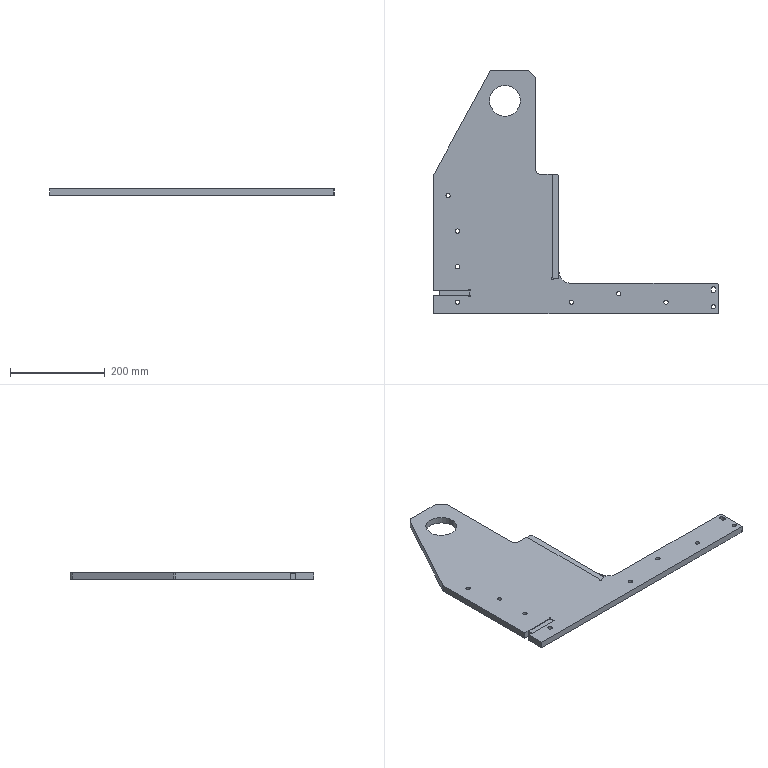Part | SolidWorks | features ICE 11, Chamfer 4, Fillet 3, Cut 1, Extrusion 1 | 1 solid | 78 faces | box 600 x 515 x 14 mm | volume 1803753 mm3 | cylinder 41 | plane 37 | commonest cylinder face diameters 9 x18 5 x13 3 x4 20 x3 65 x2 50 x1